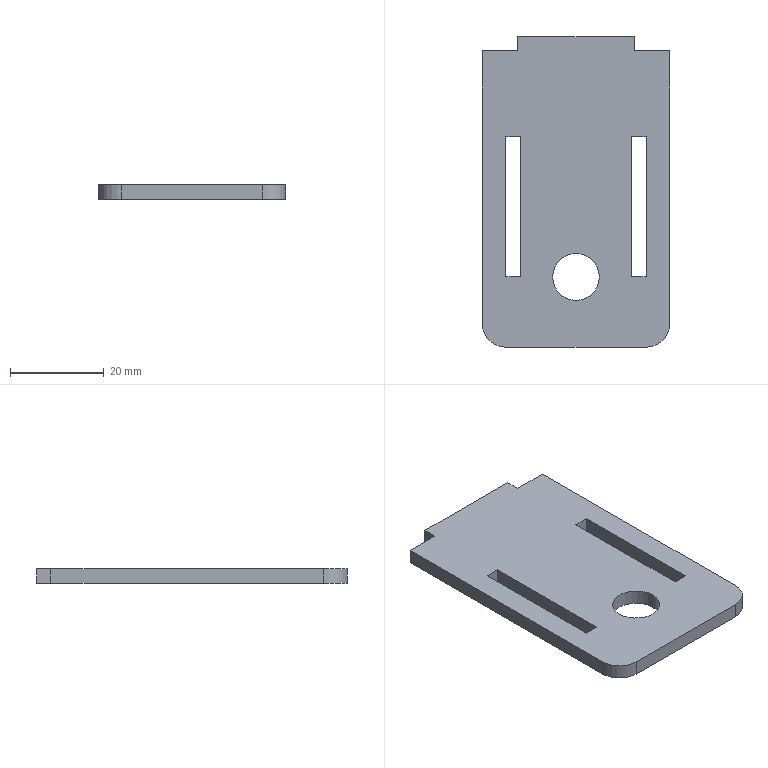Part | SolidWorks | features Fillet 1, FlatPattern 1, SMBaseFlange 1, SheetMetal 1 | 1 solid | 22 faces | box 40 x 66.3 x 3.2 mm | volume 7442 mm3 | plane 18 | cylinder 4 | commonest cylinder face diameters 10 x4
STEP:
#1=CARTESIAN_POINT('',(-5.,0.,3.2));
#2=VERTEX_POINT('',#1);
#3=CARTESIAN_POINT('',(5.,0.,3.2));
#4=VERTEX_POINT('',#3);
#5=CARTESIAN_POINT('',(0.,0.,3.2));
#6=DIRECTION('',(0.,0.,1.));
#7=DIRECTION('',(1.,0.,0.));
#8=AXIS2_PLACEMENT_3D('',#5,#6,#7);
#9=CIRCLE('',#8,5.);
#10=EDGE_CURVE('',#2,#4,#9,.T.);
#11=ORIENTED_EDGE('',*,*,#10,.T.);
#12=CARTESIAN_POINT('',(5.,0.,0.));
#13=VERTEX_POINT('',#12);
#14=CARTESIAN_POINT('',(5.,0.,3.2));
#15=DIRECTION('',(0.,0.,-1.));
#16=VECTOR('',#15,1000.);
#17=LINE('',#14,#16);
#18=EDGE_CURVE('',#4,#13,#17,.T.);
#19=ORIENTED_EDGE('',*,*,#18,.T.);
#20=CARTESIAN_POINT('',(-5.,0.,0.));
#21=VERTEX_POINT('',#20);
#22=CARTESIAN_POINT('',(0.,0.,0.));
#23=DIRECTION('',(0.,0.,1.));
#24=DIRECTION('',(1.,0.,0.));
#25=AXIS2_PLACEMENT_3D('',#22,#23,#24);
#26=CIRCLE('',#25,5.);
#27=EDGE_CURVE('',#21,#13,#26,.T.);
#28=ORIENTED_EDGE('',*,*,#27,.F.);
#29=CARTESIAN_POINT('',(-5.,0.,3.2));
#30=DIRECTION('',(0.,0.,-1.));
#31=VECTOR('',#30,1000.);
#32=LINE('',#29,#31);
#33=EDGE_CURVE('',#2,#21,#32,.T.);
#34=ORIENTED_EDGE('',*,*,#33,.F.);
#35=EDGE_LOOP('',(#11,#19,#28,#34));
#36=FACE_OUTER_BOUND('',#35,.T.);
#37=CARTESIAN_POINT('',(0.,0.,3.2));
#38=DIRECTION('',(0.,0.,-1.));
#39=DIRECTION('',(-1.,0.,0.));
#40=AXIS2_PLACEMENT_3D('',#37,#38,#39);
#41=CYLINDRICAL_SURFACE('',#40,5.);
#42=ADVANCED_FACE('',(#36),#41,.F.);
#43=CARTESIAN_POINT('',(-15.,-15.,3.2));
#44=VERTEX_POINT('',#43);
#45=CARTESIAN_POINT('',(15.,-15.,3.2));
#46=VERTEX_POINT('',#45);
#47=CARTESIAN_POINT('',(-20.,-15.,3.2));
#48=DIRECTION('',(1.,0.,0.));
#49=VECTOR('',#48,1000.);
#50=LINE('',#47,#49);
#51=EDGE_CURVE('',#44,#46,#50,.T.);
#52=ORIENTED_EDGE('',*,*,#51,.T.);
#53=CARTESIAN_POINT('',(20.,-10.,3.2));
#54=VERTEX_POINT('',#53);
#55=CARTESIAN_POINT('',(15.,-10.,3.2));
#56=DIRECTION('',(0.,0.,1.));
#57=DIRECTION('',(1.,0.,0.));
#58=AXIS2_PLACEMENT_3D('',#55,#56,#57);
#59=CIRCLE('',#58,5.);
#60=EDGE_CURVE('',#46,#54,#59,.T.);
#61=ORIENTED_EDGE('',*,*,#60,.T.);
#62=CARTESIAN_POINT('',(20.,48.3,3.2));
#63=VERTEX_POINT('',#62);
#64=CARTESIAN_POINT('',(20.,48.3,3.2));
#65=DIRECTION('',(0.,1.,0.));
#66=VECTOR('',#65,1000.);
#67=LINE('',#64,#66);
#68=EDGE_CURVE('',#54,#63,#67,.T.);
#69=ORIENTED_EDGE('',*,*,#68,.T.);
#70=CARTESIAN_POINT('',(12.5,48.3,3.2));
#71=VERTEX_POINT('',#70);
#72=CARTESIAN_POINT('',(12.5,48.3,3.2));
#73=DIRECTION('',(-1.,0.,0.));
#74=VECTOR('',#73,1000.);
#75=LINE('',#72,#74);
#76=EDGE_CURVE('',#63,#71,#75,.T.);
#77=ORIENTED_EDGE('',*,*,#76,.T.);
#78=CARTESIAN_POINT('',(12.5,51.3,3.2));
#79=VERTEX_POINT('',#78);
#80=CARTESIAN_POINT('',(12.5,48.3,3.2));
#81=DIRECTION('',(0.,1.,0.));
#82=VECTOR('',#81,1000.);
#83=LINE('',#80,#82);
#84=EDGE_CURVE('',#71,#79,#83,.T.);
#85=ORIENTED_EDGE('',*,*,#84,.T.);
#86=CARTESIAN_POINT('',(-12.5,51.3,3.2));
#87=VERTEX_POINT('',#86);
#88=CARTESIAN_POINT('',(12.5,51.3,3.2));
#89=DIRECTION('',(-1.,0.,0.));
#90=VECTOR('',#89,1000.);
#91=LINE('',#88,#90);
#92=EDGE_CURVE('',#79,#87,#91,.T.);
#93=ORIENTED_EDGE('',*,*,#92,.T.);
#94=CARTESIAN_POINT('',(-12.5,48.3,3.2));
#95=VERTEX_POINT('',#94);
#96=CARTESIAN_POINT('',(-12.5,51.3,3.2));
#97=DIRECTION('',(0.,-1.,0.));
#98=VECTOR('',#97,1000.);
#99=LINE('',#96,#98);
#100=EDGE_CURVE('',#87,#95,#99,.T.);
#101=ORIENTED_EDGE('',*,*,#100,.T.);
#102=CARTESIAN_POINT('',(-20.,48.3,3.2));
#103=VERTEX_POINT('',#102);
#104=CARTESIAN_POINT('',(-20.,48.3,3.2));
#105=DIRECTION('',(-1.,0.,0.));
#106=VECTOR('',#105,1000.);
#107=LINE('',#104,#106);
#108=EDGE_CURVE('',#95,#103,#107,.T.);
#109=ORIENTED_EDGE('',*,*,#108,.T.);
#110=CARTESIAN_POINT('',(-20.,-10.,3.2));
#111=VERTEX_POINT('',#110);
#112=CARTESIAN_POINT('',(-20.,48.3,3.2));
#113=DIRECTION('',(0.,-1.,0.));
#114=VECTOR('',#113,1000.);
#115=LINE('',#112,#114);
#116=EDGE_CURVE('',#103,#111,#115,.T.);
#117=ORIENTED_EDGE('',*,*,#116,.T.);
#118=CARTESIAN_POINT('',(-15.,-10.,3.2));
#119=DIRECTION('',(0.,0.,1.));
#120=DIRECTION('',(1.,0.,0.));
#121=AXIS2_PLACEMENT_3D('',#118,#119,#120);
#122=CIRCLE('',#121,5.);
#123=EDGE_CURVE('',#111,#44,#122,.T.);
#124=ORIENTED_EDGE('',*,*,#123,.T.);
#125=EDGE_LOOP('',(#52,#61,#69,#77,#85,#93,#101,#109,#117,#124));
#126=FACE_OUTER_BOUND('',#125,.T.);
#127=ORIENTED_EDGE('',*,*,#10,.F.);
#128=CARTESIAN_POINT('',(0.,0.,3.2));
#129=DIRECTION('',(0.,0.,1.));
#130=DIRECTION('',(1.,0.,0.));
#131=AXIS2_PLACEMENT_3D('',#128,#129,#130);
#132=CIRCLE('',#131,5.);
#133=EDGE_CURVE('',#4,#2,#132,.T.);
#134=ORIENTED_EDGE('',*,*,#133,.F.);
#135=EDGE_LOOP('',(#127,#134));
#136=FACE_BOUND('',#135,.T.);
#137=CARTESIAN_POINT('',(15.,30.,3.2));
#138=VERTEX_POINT('',#137);
#139=CARTESIAN_POINT('',(11.8,30.,3.2));
#140=VERTEX_POINT('',#139);
#141=CARTESIAN_POINT('',(15.,30.,3.2));
#142=DIRECTION('',(-1.,0.,0.));
#143=VECTOR('',#142,1000.);
#144=LINE('',#141,#143);
#145=EDGE_CURVE('',#138,#140,#144,.T.);
#146=ORIENTED_EDGE('',*,*,#145,.F.);
#147=CARTESIAN_POINT('',(15.,0.,3.2));
#148=VERTEX_POINT('',#147);
#149=CARTESIAN_POINT('',(15.,0.,3.2));
#150=DIRECTION('',(0.,1.,0.));
#151=VECTOR('',#150,1000.);
#152=LINE('',#149,#151);
#153=EDGE_CURVE('',#148,#138,#152,.T.);
#154=ORIENTED_EDGE('',*,*,#153,.F.);
#155=CARTESIAN_POINT('',(11.8,0.,3.2));
#156=VERTEX_POINT('',#155);
#157=CARTESIAN_POINT('',(15.,0.,3.2));
#158=DIRECTION('',(1.,0.,0.));
#159=VECTOR('',#158,1000.);
#160=LINE('',#157,#159);
#161=EDGE_CURVE('',#156,#148,#160,.T.);
#162=ORIENTED_EDGE('',*,*,#161,.F.);
#163=CARTESIAN_POINT('',(11.8,0.,3.2));
#164=DIRECTION('',(0.,-1.,0.));
#165=VECTOR('',#164,1000.);
#166=LINE('',#163,#165);
#167=EDGE_CURVE('',#140,#156,#166,.T.);
#168=ORIENTED_EDGE('',*,*,#167,.F.);
#169=EDGE_LOOP('',(#146,#154,#162,#168));
#170=FACE_BOUND('',#169,.T.);
#171=CARTESIAN_POINT('',(-11.8,30.,3.2));
#172=VERTEX_POINT('',#171);
#173=CARTESIAN_POINT('',(-15.,30.,3.2));
#174=VERTEX_POINT('',#173);
#175=CARTESIAN_POINT('',(-11.8,30.,3.2));
#176=DIRECTION('',(-1.,0.,0.));
#177=VECTOR('',#176,1000.);
#178=LINE('',#175,#177);
#179=EDGE_CURVE('',#172,#174,#178,.T.);
#180=ORIENTED_EDGE('',*,*,#179,.F.);
#181=CARTESIAN_POINT('',(-11.8,0.,3.2));
#182=VERTEX_POINT('',#181);
#183=CARTESIAN_POINT('',(-11.8,30.,3.2));
#184=DIRECTION('',(0.,1.,0.));
#185=VECTOR('',#184,1000.);
#186=LINE('',#183,#185);
#187=EDGE_CURVE('',#182,#172,#186,.T.);
#188=ORIENTED_EDGE('',*,*,#187,.F.);
#189=CARTESIAN_POINT('',(-15.,0.,3.2));
#190=VERTEX_POINT('',#189);
#191=CARTESIAN_POINT('',(-11.8,0.,3.2));
#192=DIRECTION('',(1.,0.,0.));
#193=VECTOR('',#192,1000.);
#194=LINE('',#191,#193);
#195=EDGE_CURVE('',#190,#182,#194,.T.);
#196=ORIENTED_EDGE('',*,*,#195,.F.);
#197=CARTESIAN_POINT('',(-15.,30.,3.2));
#198=DIRECTION('',(0.,-1.,0.));
#199=VECTOR('',#198,1000.);
#200=LINE('',#197,#199);
#201=EDGE_CURVE('',#174,#190,#200,.T.);
#202=ORIENTED_EDGE('',*,*,#201,.F.);
#203=EDGE_LOOP('',(#180,#188,#196,#202));
#204=FACE_BOUND('',#203,.T.);
#205=CARTESIAN_POINT('',(0.,0.,3.2));
#206=DIRECTION('',(0.,0.,1.));
#207=DIRECTION('',(1.,0.,0.));
#208=AXIS2_PLACEMENT_3D('',#205,#206,#207);
#209=PLANE('',#208);
#210=ADVANCED_FACE('',(#126,#136,#170,#204),#209,.T.);
#211=CARTESIAN_POINT('',(15.,0.,0.));
#212=VERTEX_POINT('',#211);
#213=CARTESIAN_POINT('',(15.,30.,0.));
#214=VERTEX_POINT('',#213);
#215=CARTESIAN_POINT('',(15.,0.,0.));
#216=DIRECTION('',(0.,1.,0.));
#217=VECTOR('',#216,1000.);
#218=LINE('',#215,#217);
#219=EDGE_CURVE('',#212,#214,#218,.T.);
#220=ORIENTED_EDGE('',*,*,#219,.T.);
#221=CARTESIAN_POINT('',(11.8,30.,0.));
#222=VERTEX_POINT('',#221);
#223=CARTESIAN_POINT('',(15.,30.,0.));
#224=DIRECTION('',(-1.,0.,0.));
#225=VECTOR('',#224,1000.);
#226=LINE('',#223,#225);
#227=EDGE_CURVE('',#214,#222,#226,.T.);
#228=ORIENTED_EDGE('',*,*,#227,.T.);
#229=CARTESIAN_POINT('',(11.8,0.,0.));
#230=VERTEX_POINT('',#229);
#231=CARTESIAN_POINT('',(11.8,0.,0.));
#232=DIRECTION('',(0.,-1.,0.));
#233=VECTOR('',#232,1000.);
#234=LINE('',#231,#233);
#235=EDGE_CURVE('',#222,#230,#234,.T.);
#236=ORIENTED_EDGE('',*,*,#235,.T.);
#237=CARTESIAN_POINT('',(15.,0.,0.));
#238=DIRECTION('',(1.,0.,0.));
#239=VECTOR('',#238,1000.);
#240=LINE('',#237,#239);
#241=EDGE_CURVE('',#230,#212,#240,.T.);
#242=ORIENTED_EDGE('',*,*,#241,.T.);
#243=EDGE_LOOP('',(#220,#228,#236,#242));
#244=FACE_BOUND('',#243,.T.);
#245=CARTESIAN_POINT('',(20.,-10.,0.));
#246=VERTEX_POINT('',#245);
#247=CARTESIAN_POINT('',(20.,48.3,0.));
#248=VERTEX_POINT('',#247);
#249=CARTESIAN_POINT('',(20.,48.3,0.));
#250=DIRECTION('',(0.,1.,0.));
#251=VECTOR('',#250,1000.);
#252=LINE('',#249,#251);
#253=EDGE_CURVE('',#246,#248,#252,.T.);
#254=ORIENTED_EDGE('',*,*,#253,.F.);
#255=CARTESIAN_POINT('',(15.,-15.,0.));
#256=VERTEX_POINT('',#255);
#257=CARTESIAN_POINT('',(15.,-10.,0.));
#258=DIRECTION('',(0.,0.,-1.));
#259=DIRECTION('',(1.,0.,0.));
#260=AXIS2_PLACEMENT_3D('',#257,#258,#259);
#261=CIRCLE('',#260,5.);
#262=EDGE_CURVE('',#246,#256,#261,.T.);
#263=ORIENTED_EDGE('',*,*,#262,.T.);
#264=CARTESIAN_POINT('',(-15.,-15.,0.));
#265=VERTEX_POINT('',#264);
#266=CARTESIAN_POINT('',(-20.,-15.,0.));
#267=DIRECTION('',(1.,0.,0.));
#268=VECTOR('',#267,1000.);
#269=LINE('',#266,#268);
#270=EDGE_CURVE('',#265,#256,#269,.T.);
#271=ORIENTED_EDGE('',*,*,#270,.F.);
#272=CARTESIAN_POINT('',(-20.,-10.,0.));
#273=VERTEX_POINT('',#272);
#274=CARTESIAN_POINT('',(-15.,-10.,0.));
#275=DIRECTION('',(0.,0.,-1.));
#276=DIRECTION('',(1.,0.,0.));
#277=AXIS2_PLACEMENT_3D('',#274,#275,#276);
#278=CIRCLE('',#277,5.);
#279=EDGE_CURVE('',#265,#273,#278,.T.);
#280=ORIENTED_EDGE('',*,*,#279,.T.);
#281=CARTESIAN_POINT('',(-20.,48.3,0.));
#282=VERTEX_POINT('',#281);
#283=CARTESIAN_POINT('',(-20.,48.3,0.));
#284=DIRECTION('',(0.,-1.,0.));
#285=VECTOR('',#284,1000.);
#286=LINE('',#283,#285);
#287=EDGE_CURVE('',#282,#273,#286,.T.);
#288=ORIENTED_EDGE('',*,*,#287,.F.);
#289=CARTESIAN_POINT('',(-12.5,48.3,0.));
#290=VERTEX_POINT('',#289);
#291=CARTESIAN_POINT('',(-20.,48.3,0.));
#292=DIRECTION('',(-1.,0.,0.));
#293=VECTOR('',#292,1000.);
#294=LINE('',#291,#293);
#295=EDGE_CURVE('',#290,#282,#294,.T.);
#296=ORIENTED_EDGE('',*,*,#295,.F.);
#297=CARTESIAN_POINT('',(-12.5,51.3,0.));
#298=VERTEX_POINT('',#297);
#299=CARTESIAN_POINT('',(-12.5,51.3,0.));
#300=DIRECTION('',(0.,-1.,0.));
#301=VECTOR('',#300,1000.);
#302=LINE('',#299,#301);
#303=EDGE_CURVE('',#298,#290,#302,.T.);
#304=ORIENTED_EDGE('',*,*,#303,.F.);
#305=CARTESIAN_POINT('',(12.5,51.3,0.));
#306=VERTEX_POINT('',#305);
#307=CARTESIAN_POINT('',(12.5,51.3,0.));
#308=DIRECTION('',(-1.,0.,0.));
#309=VECTOR('',#308,1000.);
#310=LINE('',#307,#309);
#311=EDGE_CURVE('',#306,#298,#310,.T.);
#312=ORIENTED_EDGE('',*,*,#311,.F.);
#313=CARTESIAN_POINT('',(12.5,48.3,0.));
#314=VERTEX_POINT('',#313);
#315=CARTESIAN_POINT('',(12.5,48.3,0.));
#316=DIRECTION('',(0.,1.,0.));
#317=VECTOR('',#316,1000.);
#318=LINE('',#315,#317);
#319=EDGE_CURVE('',#314,#306,#318,.T.);
#320=ORIENTED_EDGE('',*,*,#319,.F.);
#321=CARTESIAN_POINT('',(12.5,48.3,0.));
#322=DIRECTION('',(-1.,0.,0.));
#323=VECTOR('',#322,1000.);
#324=LINE('',#321,#323);
#325=EDGE_CURVE('',#248,#314,#324,.T.);
#326=ORIENTED_EDGE('',*,*,#325,.F.);
#327=EDGE_LOOP('',(#254,#263,#271,#280,#288,#296,#304,#312,#320,#326));
#328=FACE_OUTER_BOUND('',#327,.T.);
#329=ORIENTED_EDGE('',*,*,#27,.T.);
#330=CARTESIAN_POINT('',(0.,0.,0.));
#331=DIRECTION('',(0.,0.,1.));
#332=DIRECTION('',(1.,0.,0.));
#333=AXIS2_PLACEMENT_3D('',#330,#331,#332);
#334=CIRCLE('',#333,5.);
#335=EDGE_CURVE('',#13,#21,#334,.T.);
#336=ORIENTED_EDGE('',*,*,#335,.T.);
#337=EDGE_LOOP('',(#329,#336));
#338=FACE_BOUND('',#337,.T.);
#339=CARTESIAN_POINT('',(-11.8,0.,0.));
#340=VERTEX_POINT('',#339);
#341=CARTESIAN_POINT('',(-11.8,30.,0.));
#342=VERTEX_POINT('',#341);
#343=CARTESIAN_POINT('',(-11.8,30.,0.));
#344=DIRECTION('',(0.,1.,0.));
#345=VECTOR('',#344,1000.);
#346=LINE('',#343,#345);
#347=EDGE_CURVE('',#340,#342,#346,.T.);
#348=ORIENTED_EDGE('',*,*,#347,.T.);
#349=CARTESIAN_POINT('',(-15.,30.,0.));
#350=VERTEX_POINT('',#349);
#351=CARTESIAN_POINT('',(-11.8,30.,0.));
#352=DIRECTION('',(-1.,0.,0.));
#353=VECTOR('',#352,1000.);
#354=LINE('',#351,#353);
#355=EDGE_CURVE('',#342,#350,#354,.T.);
#356=ORIENTED_EDGE('',*,*,#355,.T.);
#357=CARTESIAN_POINT('',(-15.,0.,0.));
#358=VERTEX_POINT('',#357);
#359=CARTESIAN_POINT('',(-15.,30.,0.));
#360=DIRECTION('',(0.,-1.,0.));
#361=VECTOR('',#360,1000.);
#362=LINE('',#359,#361);
#363=EDGE_CURVE('',#350,#358,#362,.T.);
#364=ORIENTED_EDGE('',*,*,#363,.T.);
#365=CARTESIAN_POINT('',(-11.8,0.,0.));
#366=DIRECTION('',(1.,0.,0.));
#367=VECTOR('',#366,1000.);
#368=LINE('',#365,#367);
#369=EDGE_CURVE('',#358,#340,#368,.T.);
#370=ORIENTED_EDGE('',*,*,#369,.T.);
#371=EDGE_LOOP('',(#348,#356,#364,#370));
#372=FACE_BOUND('',#371,.T.);
#373=CARTESIAN_POINT('',(0.,0.,0.));
#374=DIRECTION('',(0.,0.,1.));
#375=DIRECTION('',(1.,0.,0.));
#376=AXIS2_PLACEMENT_3D('',#373,#374,#375);
#377=PLANE('',#376);
#378=ADVANCED_FACE('',(#244,#328,#338,#372),#377,.F.);
#379=ORIENTED_EDGE('',*,*,#287,.T.);
#380=CARTESIAN_POINT('',(-20.,-10.,3.2));
#381=DIRECTION('',(0.,0.,1.));
#382=VECTOR('',#381,1000.);
#383=LINE('',#380,#382);
#384=EDGE_CURVE('',#273,#111,#383,.T.);
#385=ORIENTED_EDGE('',*,*,#384,.T.);
#386=ORIENTED_EDGE('',*,*,#116,.F.);
#387=CARTESIAN_POINT('',(-20.,48.3,3.2));
#388=DIRECTION('',(0.,0.,-1.));
#389=VECTOR('',#388,1000.);
#390=LINE('',#387,#389);
#391=EDGE_CURVE('',#103,#282,#390,.T.);
#392=ORIENTED_EDGE('',*,*,#391,.T.);
#393=EDGE_LOOP('',(#379,#385,#386,#392));
#394=FACE_OUTER_BOUND('',#393,.T.);
#395=CARTESIAN_POINT('',(-20.,48.3,3.2));
#396=DIRECTION('',(1.,0.,0.));
#397=DIRECTION('',(0.,1.,0.));
#398=AXIS2_PLACEMENT_3D('',#395,#396,#397);
#399=PLANE('',#398);
#400=ADVANCED_FACE('',(#394),#399,.F.);
#401=ORIENTED_EDGE('',*,*,#270,.T.);
#402=CARTESIAN_POINT('',(15.,-15.,3.2));
#403=DIRECTION('',(0.,0.,1.));
#404=VECTOR('',#403,1000.);
#405=LINE('',#402,#404);
#406=EDGE_CURVE('',#256,#46,#405,.T.);
#407=ORIENTED_EDGE('',*,*,#406,.T.);
#408=ORIENTED_EDGE('',*,*,#51,.F.);
#409=CARTESIAN_POINT('',(-15.,-15.,3.2));
#410=DIRECTION('',(0.,0.,-1.));
#411=VECTOR('',#410,1000.);
#412=LINE('',#409,#411);
#413=EDGE_CURVE('',#44,#265,#412,.T.);
#414=ORIENTED_EDGE('',*,*,#413,.T.);
#415=EDGE_LOOP('',(#401,#407,#408,#414));
#416=FACE_OUTER_BOUND('',#415,.T.);
#417=CARTESIAN_POINT('',(-20.,-15.,3.2));
#418=DIRECTION('',(0.,1.,0.));
#419=DIRECTION('',(0.,0.,1.));
#420=AXIS2_PLACEMENT_3D('',#417,#418,#419);
#421=PLANE('',#420);
#422=ADVANCED_FACE('',(#416),#421,.F.);
#423=ORIENTED_EDGE('',*,*,#68,.F.);
#424=CARTESIAN_POINT('',(20.,-10.,3.2));
#425=DIRECTION('',(0.,0.,-1.));
#426=VECTOR('',#425,1000.);
#427=LINE('',#424,#426);
#428=EDGE_CURVE('',#54,#246,#427,.T.);
#429=ORIENTED_EDGE('',*,*,#428,.T.);
#430=ORIENTED_EDGE('',*,*,#253,.T.);
#431=CARTESIAN_POINT('',(20.,48.3,3.2));
#432=DIRECTION('',(0.,0.,-1.));
#433=VECTOR('',#432,1000.);
#434=LINE('',#431,#433);
#435=EDGE_CURVE('',#63,#248,#434,.T.);
#436=ORIENTED_EDGE('',*,*,#435,.F.);
#437=EDGE_LOOP('',(#423,#429,#430,#436));
#438=FACE_OUTER_BOUND('',#437,.T.);
#439=CARTESIAN_POINT('',(20.,48.3,3.2));
#440=DIRECTION('',(-1.,0.,0.));
#441=DIRECTION('',(0.,-1.,0.));
#442=AXIS2_PLACEMENT_3D('',#439,#440,#441);
#443=PLANE('',#442);
#444=ADVANCED_FACE('',(#438),#443,.F.);
#445=ORIENTED_EDGE('',*,*,#325,.T.);
#446=CARTESIAN_POINT('',(12.5,48.3,3.2));
#447=DIRECTION('',(0.,0.,-1.));
#448=VECTOR('',#447,1000.);
#449=LINE('',#446,#448);
#450=EDGE_CURVE('',#71,#314,#449,.T.);
#451=ORIENTED_EDGE('',*,*,#450,.F.);
#452=ORIENTED_EDGE('',*,*,#76,.F.);
#453=ORIENTED_EDGE('',*,*,#435,.T.);
#454=EDGE_LOOP('',(#445,#451,#452,#453));
#455=FACE_OUTER_BOUND('',#454,.T.);
#456=CARTESIAN_POINT('',(12.5,48.3,3.2));
#457=DIRECTION('',(0.,-1.,0.));
#458=DIRECTION('',(0.,0.,-1.));
#459=AXIS2_PLACEMENT_3D('',#456,#457,#458);
#460=PLANE('',#459);
#461=ADVANCED_FACE('',(#455),#460,.F.);
#462=ORIENTED_EDGE('',*,*,#319,.T.);
#463=CARTESIAN_POINT('',(12.5,51.3,3.2));
#464=DIRECTION('',(0.,0.,-1.));
#465=VECTOR('',#464,1000.);
#466=LINE('',#463,#465);
#467=EDGE_CURVE('',#79,#306,#466,.T.);
#468=ORIENTED_EDGE('',*,*,#467,.F.);
#469=ORIENTED_EDGE('',*,*,#84,.F.);
#470=ORIENTED_EDGE('',*,*,#450,.T.);
#471=EDGE_LOOP('',(#462,#468,#469,#470));
#472=FACE_OUTER_BOUND('',#471,.T.);
#473=CARTESIAN_POINT('',(12.5,48.3,3.2));
#474=DIRECTION('',(-1.,0.,0.));
#475=DIRECTION('',(0.,0.,1.));
#476=AXIS2_PLACEMENT_3D('',#473,#474,#475);
#477=PLANE('',#476);
#478=ADVANCED_FACE('',(#472),#477,.F.);
#479=ORIENTED_EDGE('',*,*,#311,.T.);
#480=CARTESIAN_POINT('',(-12.5,51.3,3.2));
#481=DIRECTION('',(0.,0.,-1.));
#482=VECTOR('',#481,1000.);
#483=LINE('',#480,#482);
#484=EDGE_CURVE('',#87,#298,#483,.T.);
#485=ORIENTED_EDGE('',*,*,#484,.F.);
#486=ORIENTED_EDGE('',*,*,#92,.F.);
#487=ORIENTED_EDGE('',*,*,#467,.T.);
#488=EDGE_LOOP('',(#479,#485,#486,#487));
#489=FACE_OUTER_BOUND('',#488,.T.);
#490=CARTESIAN_POINT('',(12.5,51.3,3.2));
#491=DIRECTION('',(0.,-1.,0.));
#492=DIRECTION('',(0.,0.,-1.));
#493=AXIS2_PLACEMENT_3D('',#490,#491,#492);
#494=PLANE('',#493);
#495=ADVANCED_FACE('',(#489),#494,.F.);
#496=ORIENTED_EDGE('',*,*,#303,.T.);
#497=CARTESIAN_POINT('',(-12.5,48.3,3.2));
#498=DIRECTION('',(0.,0.,-1.));
#499=VECTOR('',#498,1000.);
#500=LINE('',#497,#499);
#501=EDGE_CURVE('',#95,#290,#500,.T.);
#502=ORIENTED_EDGE('',*,*,#501,.F.);
#503=ORIENTED_EDGE('',*,*,#100,.F.);
#504=ORIENTED_EDGE('',*,*,#484,.T.);
#505=EDGE_LOOP('',(#496,#502,#503,#504));
#506=FACE_OUTER_BOUND('',#505,.T.);
#507=CARTESIAN_POINT('',(-12.5,51.3,3.2));
#508=DIRECTION('',(1.,0.,0.));
#509=DIRECTION('',(0.,0.,-1.));
#510=AXIS2_PLACEMENT_3D('',#507,#508,#509);
#511=PLANE('',#510);
#512=ADVANCED_FACE('',(#506),#511,.F.);
#513=ORIENTED_EDGE('',*,*,#295,.T.);
#514=ORIENTED_EDGE('',*,*,#391,.F.);
#515=ORIENTED_EDGE('',*,*,#108,.F.);
#516=ORIENTED_EDGE('',*,*,#501,.T.);
#517=EDGE_LOOP('',(#513,#514,#515,#516));
#518=FACE_OUTER_BOUND('',#517,.T.);
#519=CARTESIAN_POINT('',(-20.,48.3,3.2));
#520=DIRECTION('',(0.,-1.,0.));
#521=DIRECTION('',(0.,0.,-1.));
#522=AXIS2_PLACEMENT_3D('',#519,#520,#521);
#523=PLANE('',#522);
#524=ADVANCED_FACE('',(#518),#523,.F.);
#525=ORIENTED_EDGE('',*,*,#18,.F.);
#526=ORIENTED_EDGE('',*,*,#133,.T.);
#527=ORIENTED_EDGE('',*,*,#33,.T.);
#528=ORIENTED_EDGE('',*,*,#335,.F.);
#529=EDGE_LOOP('',(#525,#526,#527,#528));
#530=FACE_OUTER_BOUND('',#529,.T.);
#531=CARTESIAN_POINT('',(0.,0.,3.2));
#532=DIRECTION('',(0.,0.,-1.));
#533=DIRECTION('',(-1.,0.,0.));
#534=AXIS2_PLACEMENT_3D('',#531,#532,#533);
#535=CYLINDRICAL_SURFACE('',#534,5.);
#536=ADVANCED_FACE('',(#530),#535,.F.);
#537=ORIENTED_EDGE('',*,*,#219,.F.);
#538=CARTESIAN_POINT('',(15.,0.,3.2));
#539=DIRECTION('',(0.,0.,-1.));
#540=VECTOR('',#539,1000.);
#541=LINE('',#538,#540);
#542=EDGE_CURVE('',#148,#212,#541,.T.);
#543=ORIENTED_EDGE('',*,*,#542,.F.);
#544=ORIENTED_EDGE('',*,*,#153,.T.);
#545=CARTESIAN_POINT('',(15.,30.,3.2));
#546=DIRECTION('',(0.,0.,-1.));
#547=VECTOR('',#546,1000.);
#548=LINE('',#545,#547);
#549=EDGE_CURVE('',#138,#214,#548,.T.);
#550=ORIENTED_EDGE('',*,*,#549,.T.);
#551=EDGE_LOOP('',(#537,#543,#544,#550));
#552=FACE_OUTER_BOUND('',#551,.T.);
#553=CARTESIAN_POINT('',(15.,0.,3.2));
#554=DIRECTION('',(-1.,0.,0.));
#555=DIRECTION('',(0.,0.,1.));
#556=AXIS2_PLACEMENT_3D('',#553,#554,#555);
#557=PLANE('',#556);
#558=ADVANCED_FACE('',(#552),#557,.T.);
#559=ORIENTED_EDGE('',*,*,#227,.F.);
#560=ORIENTED_EDGE('',*,*,#549,.F.);
#561=ORIENTED_EDGE('',*,*,#145,.T.);
#562=CARTESIAN_POINT('',(11.8,30.,3.2));
#563=DIRECTION('',(0.,0.,-1.));
#564=VECTOR('',#563,1000.);
#565=LINE('',#562,#564);
#566=EDGE_CURVE('',#140,#222,#565,.T.);
#567=ORIENTED_EDGE('',*,*,#566,.T.);
#568=EDGE_LOOP('',(#559,#560,#561,#567));
#569=FACE_OUTER_BOUND('',#568,.T.);
#570=CARTESIAN_POINT('',(15.,30.,3.2));
#571=DIRECTION('',(0.,-1.,0.));
#572=DIRECTION('',(1.,0.,0.));
#573=AXIS2_PLACEMENT_3D('',#570,#571,#572);
#574=PLANE('',#573);
#575=ADVANCED_FACE('',(#569),#574,.T.);
#576=ORIENTED_EDGE('',*,*,#235,.F.);
#577=ORIENTED_EDGE('',*,*,#566,.F.);
#578=ORIENTED_EDGE('',*,*,#167,.T.);
#579=CARTESIAN_POINT('',(11.8,0.,3.2));
#580=DIRECTION('',(0.,0.,-1.));
#581=VECTOR('',#580,1000.);
#582=LINE('',#579,#581);
#583=EDGE_CURVE('',#156,#230,#582,.T.);
#584=ORIENTED_EDGE('',*,*,#583,.T.);
#585=EDGE_LOOP('',(#576,#577,#578,#584));
#586=FACE_OUTER_BOUND('',#585,.T.);
#587=CARTESIAN_POINT('',(11.8,0.,3.2));
#588=DIRECTION('',(1.,0.,0.));
#589=DIRECTION('',(0.,0.,-1.));
#590=AXIS2_PLACEMENT_3D('',#587,#588,#589);
#591=PLANE('',#590);
#592=ADVANCED_FACE('',(#586),#591,.T.);
#593=ORIENTED_EDGE('',*,*,#241,.F.);
#594=ORIENTED_EDGE('',*,*,#583,.F.);
#595=ORIENTED_EDGE('',*,*,#161,.T.);
#596=ORIENTED_EDGE('',*,*,#542,.T.);
#597=EDGE_LOOP('',(#593,#594,#595,#596));
#598=FACE_OUTER_BOUND('',#597,.T.);
#599=CARTESIAN_POINT('',(15.,0.,3.2));
#600=DIRECTION('',(0.,1.,0.));
#601=DIRECTION('',(-1.,0.,0.));
#602=AXIS2_PLACEMENT_3D('',#599,#600,#601);
#603=PLANE('',#602);
#604=ADVANCED_FACE('',(#598),#603,.T.);
#605=ORIENTED_EDGE('',*,*,#347,.F.);
#606=CARTESIAN_POINT('',(-11.8,0.,3.2));
#607=DIRECTION('',(0.,0.,-1.));
#608=VECTOR('',#607,1000.);
#609=LINE('',#606,#608);
#610=EDGE_CURVE('',#182,#340,#609,.T.);
#611=ORIENTED_EDGE('',*,*,#610,.F.);
#612=ORIENTED_EDGE('',*,*,#187,.T.);
#613=CARTESIAN_POINT('',(-11.8,30.,3.2));
#614=DIRECTION('',(0.,0.,-1.));
#615=VECTOR('',#614,1000.);
#616=LINE('',#613,#615);
#617=EDGE_CURVE('',#172,#342,#616,.T.);
#618=ORIENTED_EDGE('',*,*,#617,.T.);
#619=EDGE_LOOP('',(#605,#611,#612,#618));
#620=FACE_OUTER_BOUND('',#619,.T.);
#621=CARTESIAN_POINT('',(-11.8,30.,3.2));
#622=DIRECTION('',(-1.,0.,0.));
#623=DIRECTION('',(0.,-1.,0.));
#624=AXIS2_PLACEMENT_3D('',#621,#622,#623);
#625=PLANE('',#624);
#626=ADVANCED_FACE('',(#620),#625,.T.);
#627=ORIENTED_EDGE('',*,*,#355,.F.);
#628=ORIENTED_EDGE('',*,*,#617,.F.);
#629=ORIENTED_EDGE('',*,*,#179,.T.);
#630=CARTESIAN_POINT('',(-15.,30.,3.2));
#631=DIRECTION('',(0.,0.,-1.));
#632=VECTOR('',#631,1000.);
#633=LINE('',#630,#632);
#634=EDGE_CURVE('',#174,#350,#633,.T.);
#635=ORIENTED_EDGE('',*,*,#634,.T.);
#636=EDGE_LOOP('',(#627,#628,#629,#635));
#637=FACE_OUTER_BOUND('',#636,.T.);
#638=CARTESIAN_POINT('',(-11.8,30.,3.2));
#639=DIRECTION('',(0.,-1.,0.));
#640=DIRECTION('',(0.,0.,-1.));
#641=AXIS2_PLACEMENT_3D('',#638,#639,#640);
#642=PLANE('',#641);
#643=ADVANCED_FACE('',(#637),#642,.T.);
#644=ORIENTED_EDGE('',*,*,#363,.F.);
#645=ORIENTED_EDGE('',*,*,#634,.F.);
#646=ORIENTED_EDGE('',*,*,#201,.T.);
#647=CARTESIAN_POINT('',(-15.,0.,3.2));
#648=DIRECTION('',(0.,0.,-1.));
#649=VECTOR('',#648,1000.);
#650=LINE('',#647,#649);
#651=EDGE_CURVE('',#190,#358,#650,.T.);
#652=ORIENTED_EDGE('',*,*,#651,.T.);
#653=EDGE_LOOP('',(#644,#645,#646,#652));
#654=FACE_OUTER_BOUND('',#653,.T.);
#655=CARTESIAN_POINT('',(-15.,30.,3.2));
#656=DIRECTION('',(1.,0.,0.));
#657=DIRECTION('',(0.,1.,0.));
#658=AXIS2_PLACEMENT_3D('',#655,#656,#657);
#659=PLANE('',#658);
#660=ADVANCED_FACE('',(#654),#659,.T.);
#661=ORIENTED_EDGE('',*,*,#369,.F.);
#662=ORIENTED_EDGE('',*,*,#651,.F.);
#663=ORIENTED_EDGE('',*,*,#195,.T.);
#664=ORIENTED_EDGE('',*,*,#610,.T.);
#665=EDGE_LOOP('',(#661,#662,#663,#664));
#666=FACE_OUTER_BOUND('',#665,.T.);
#667=CARTESIAN_POINT('',(-11.8,0.,3.2));
#668=DIRECTION('',(0.,1.,0.));
#669=DIRECTION('',(-1.,0.,0.));
#670=AXIS2_PLACEMENT_3D('',#667,#668,#669);
#671=PLANE('',#670);
#672=ADVANCED_FACE('',(#666),#671,.T.);
#673=ORIENTED_EDGE('',*,*,#60,.F.);
#674=ORIENTED_EDGE('',*,*,#406,.F.);
#675=ORIENTED_EDGE('',*,*,#262,.F.);
#676=ORIENTED_EDGE('',*,*,#428,.F.);
#677=EDGE_LOOP('',(#673,#674,#675,#676));
#678=FACE_OUTER_BOUND('',#677,.T.);
#679=CARTESIAN_POINT('',(15.,-10.,3.2));
#680=DIRECTION('',(0.,0.,-1.));
#681=DIRECTION('',(-1.,0.,0.));
#682=AXIS2_PLACEMENT_3D('',#679,#680,#681);
#683=CYLINDRICAL_SURFACE('',#682,5.);
#684=ADVANCED_FACE('',(#678),#683,.T.);
#685=ORIENTED_EDGE('',*,*,#123,.F.);
#686=ORIENTED_EDGE('',*,*,#384,.F.);
#687=ORIENTED_EDGE('',*,*,#279,.F.);
#688=ORIENTED_EDGE('',*,*,#413,.F.);
#689=EDGE_LOOP('',(#685,#686,#687,#688));
#690=FACE_OUTER_BOUND('',#689,.T.);
#691=CARTESIAN_POINT('',(-15.,-10.,3.2));
#692=DIRECTION('',(0.,0.,-1.));
#693=DIRECTION('',(-1.,0.,0.));
#694=AXIS2_PLACEMENT_3D('',#691,#692,#693);
#695=CYLINDRICAL_SURFACE('',#694,5.);
#696=ADVANCED_FACE('',(#690),#695,.T.);
#697=CLOSED_SHELL('',(#42,#210,#378,#400,#422,#444,#461,#478,#495,#512,#524,#536,#558,#575,#592,#604,#626,#643,#660,#672,#684,#696));
#698=MANIFOLD_SOLID_BREP('',#697);
#699=CARTESIAN_POINT('',(0.,0.,0.));
#700=DIRECTION('',(0.,0.,1.));
#701=DIRECTION('',(1.,0.,0.));
#702=AXIS2_PLACEMENT_3D('',#699,#700,#701);
#703=(LENGTH_UNIT()NAMED_UNIT(*)SI_UNIT(.MILLI.,.METRE.));
#704=UNCERTAINTY_MEASURE_WITH_UNIT(LENGTH_MEASURE(0.00001),#703,'','');
#705=(NAMED_UNIT(*)PLANE_ANGLE_UNIT()SI_UNIT($,.RADIAN.));
#706=(NAMED_UNIT(*)SI_UNIT($,.STERADIAN.)SOLID_ANGLE_UNIT());
#707=(GEOMETRIC_REPRESENTATION_CONTEXT(3)GLOBAL_UNCERTAINTY_ASSIGNED_CONTEXT((#704))GLOBAL_UNIT_ASSIGNED_CONTEXT((#703,#705,#706))REPRESENTATION_CONTEXT('',''));
#708=ADVANCED_BREP_SHAPE_REPRESENTATION('',(#698,#702),#707);